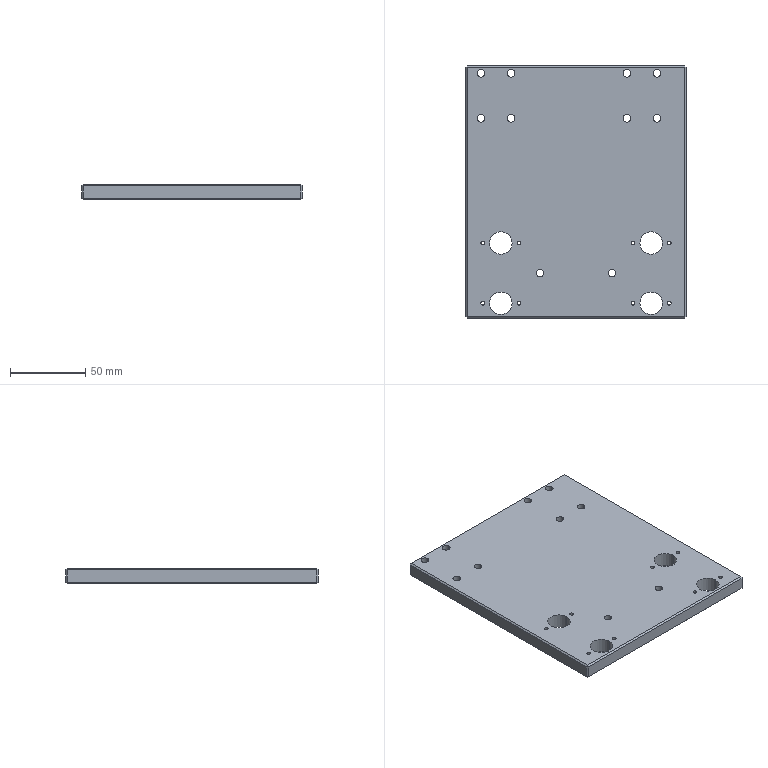Part | STEP file | 04-17 pre-press fixing plate | 1 solid | 70 faces | box 146.4 x 168 x 10 mm | volume 235820 mm3 | cylinder 44 | plane 26 | commonest cylinder face diameters 2.5 x16 5.1 x16 15 x8 5 x4